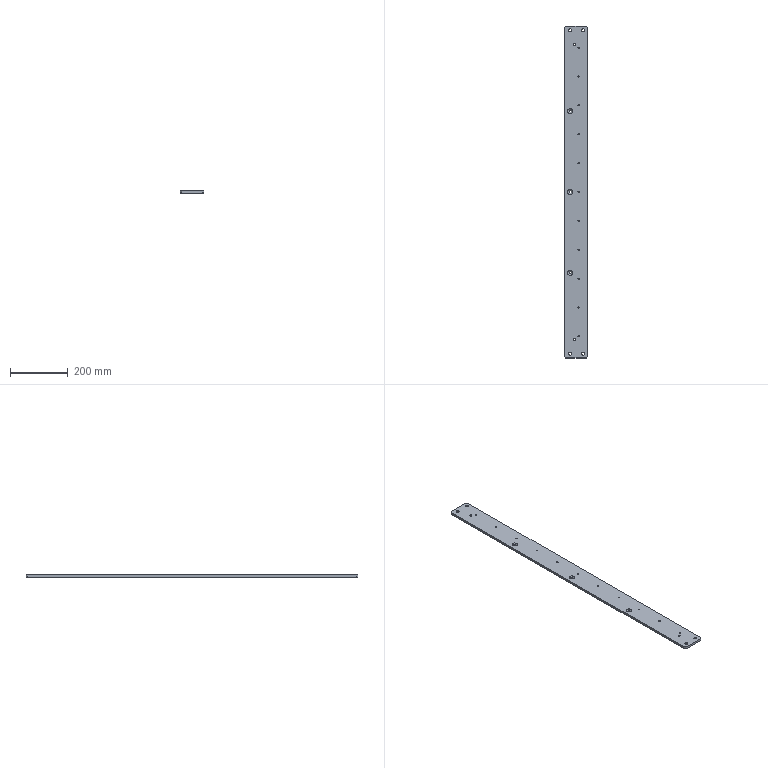Part | NX | features BREP 1 | 1 solid | 64 faces | box 80 x 1150 x 8 mm | volume 728047 mm3 | cylinder 40 | cone 14 | plane 10 | commonest cylinder face diameters 4.2 x22 10 x8 9 x6 6.8 x4